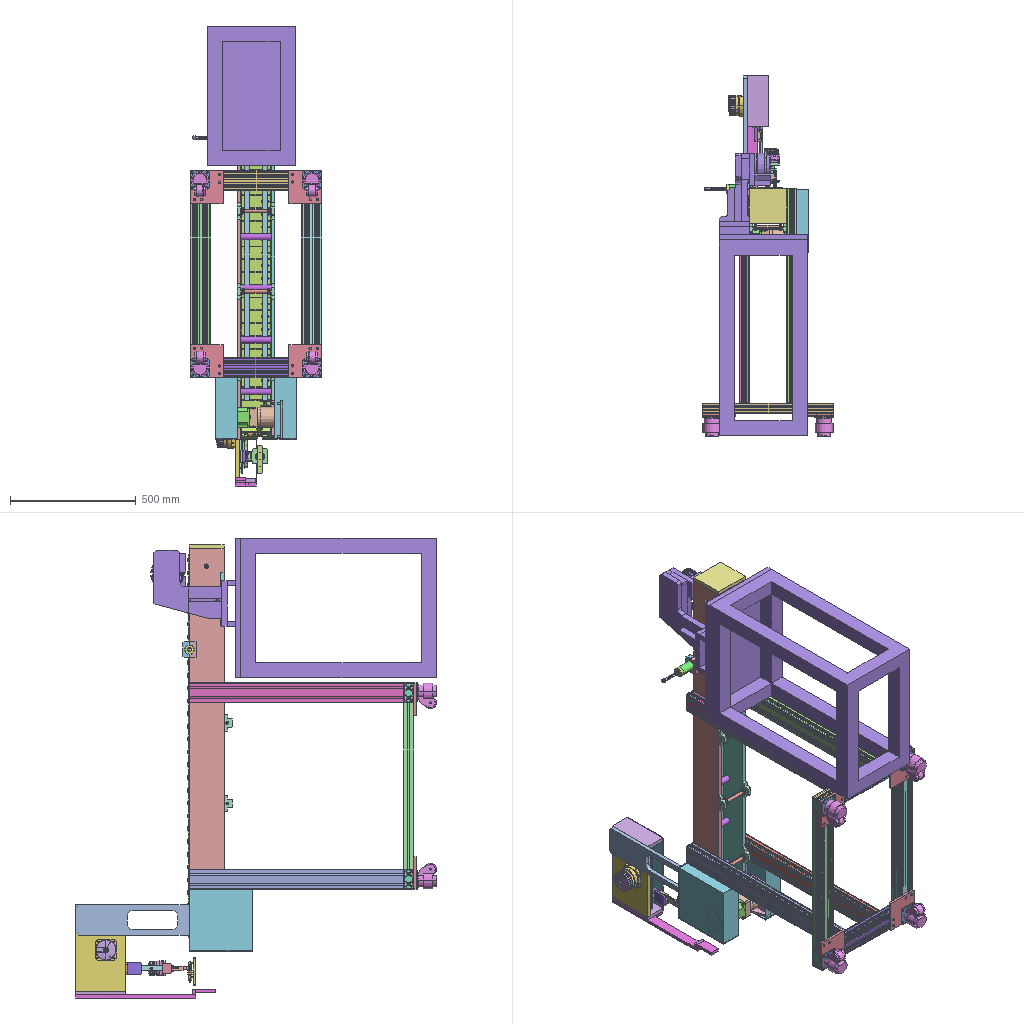Assembly | STEP file | 68 different items | 200 placed | box 524 x 1433 x 1827 mm
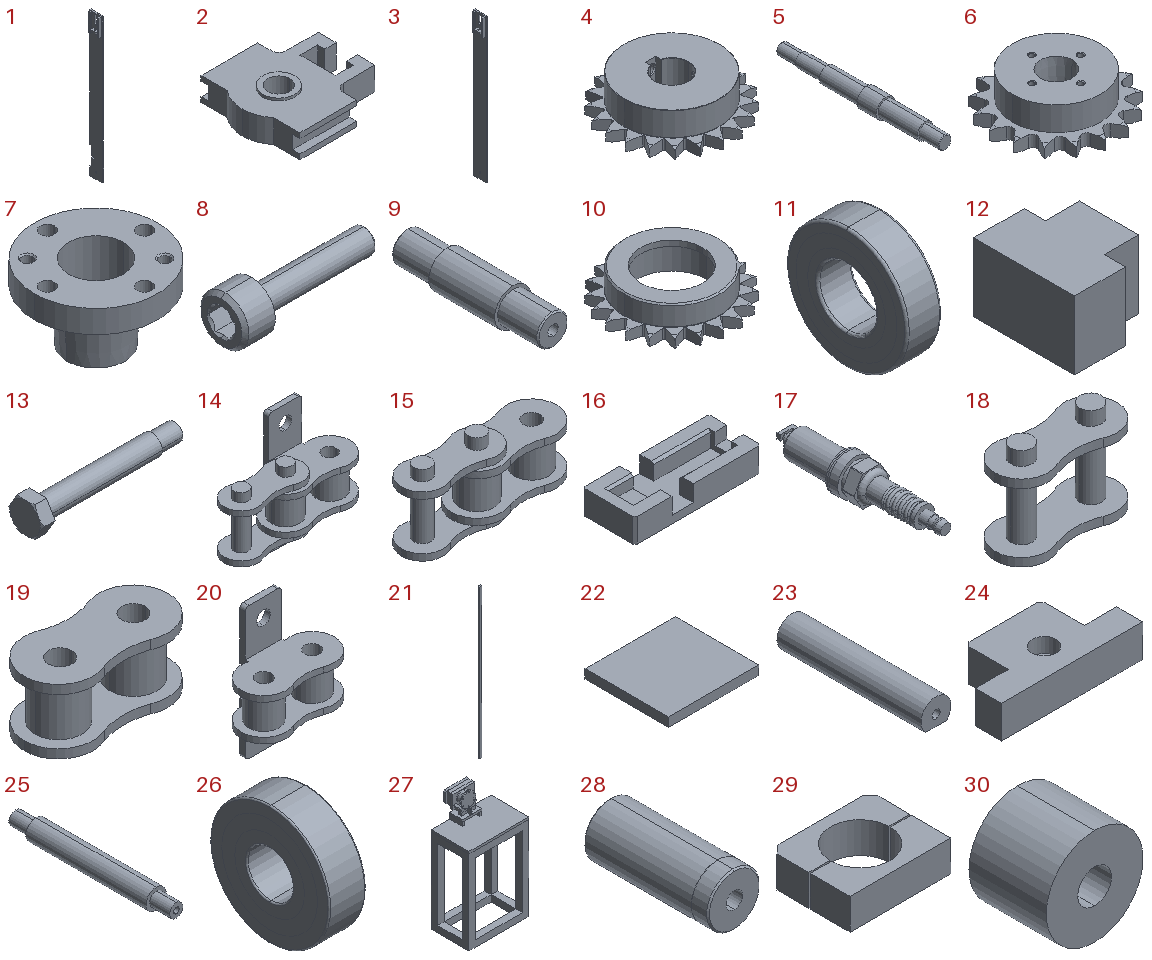Parts list (item | name | quantity | parent item | size | volume):
1 | PN_0020 | x1 | - | 50 x 139 x 1600 mm | 3436426 mm3
2 | UCT204 | x2 | - | 94 x 89 x 31 mm | 112461 mm3
3 | PN_0012 | x1 | - | 50 x 139 x 1600 mm | 3495566 mm3
4 | SP40B21_N_25_SP40B21-N-25 | x2 | - | 91.743 x 91.486 x 25 mm | 93110 mm3
5 | PN_0021 | x1 | - | 30 x 255 x 30 mm | 110798 mm3
6 | LFSP40B17_17_Asp | x2 | in LFSP40B17_17_A_LFSP40B17-17-A | 75.676 x 75.353 x 22 mm | 51808 mm3
7 | LFSP35B_17_boltbushing | x2 | in LFSP40B17_17_A_LFSP40B17-17-A | 38 x 38 x 23 mm | 6598 mm3
8 | LFSP35B17boltbolt | x8 | in LFSP40B17_17_A_LFSP40B17-17-A | 24 x 8 x 8 mm | 437.542 mm3
9 | PN_0023 | x1 | - | 30 x 120 x 30 mm | 67614 mm3
10 | PN_0022_SP40B21-N-25 | x2 | - | 91.743 x 91.486 x 22 mm | 50734 mm3
11 | 6205ZZ series deep groove ball bearing_6205ZZ | x2 | - | 15 x 52 x 52 mm | 22330 mm3
12 | PN_0024 | x2 | - | 26 x 31 x 21 mm | 12363 mm3
13 | PN_0025_M14x95 | x2 | - | 103.8 x 24.249 x 21 mm | 17342 mm3
14 | CHEL40Achain | x6 | in CHEL40A_4_CHEL40A-4 | 36.1 x 13.75 x 34.8 mm | 2522 mm3
15 | CHEL40Achain-2 | x4 | in CHEL40A_4_CHEL40A-4 | 36.1 x 11.7 x 17.55 mm | 2131 mm3
16 | PN_0002 | x33 | in PN_0001 | 116 x 48 x 22 mm | 82271 mm3
17 | FR8SES | x36 | in PN_0001, Assembly 2, PN_0030, PN_0045 | 18.6 x 85.1 x 18.6 mm | 9845 mm3
18 | CHEL40Achain-3 | x4 | - | 22.4 x 9.7 x 17.55 mm | 895.476 mm3
19 | CHEL40Achain-4 | x2 | - | 24.4 x 11.7 x 10.95 mm | 1235 mm3
20 | CHEL40Achain-5 | x2 | - | 24.4 x 13.75 x 34.8 mm | 1627 mm3
21 | PN_0026 | x2 | - | 20 x 16 x 1290 mm | 377295 mm3
22 | PN_0004 | x1 | - | 150 x 139 x 15 mm | 312750 mm3
23 | PN_0003 | x5 | - | 25 x 120 x 21.5 mm | 52408 mm3
24 | PN_0005 | x6 | - | 65 x 32 x 15 mm | 21213 mm3
25 | PN_0006 | x3 | - | 15 x 120 x 15 mm | 17905 mm3
26 | 6000ZZ series deep groove ball bearing_6000ZZ | x6 | - | 8 x 26 x 26 mm | 3330 mm3
27 | Wire-arranging machine schematic | x1 | in Assembly 2 | 555 x 350.2 x 1135 mm | 27799243 mm3
28 | PN_0007 | x1 | in PN_0027 | 38 x 97.6 x 38 mm | 92613 mm3
29 | PN_0008 | x1 | in PN_0027 | 65 x 52 x 20 mm | 43878 mm3
30 | PN_0011 | x1 | in PN_0027 | 10 x 8 x 10 mm | 476.737 mm3
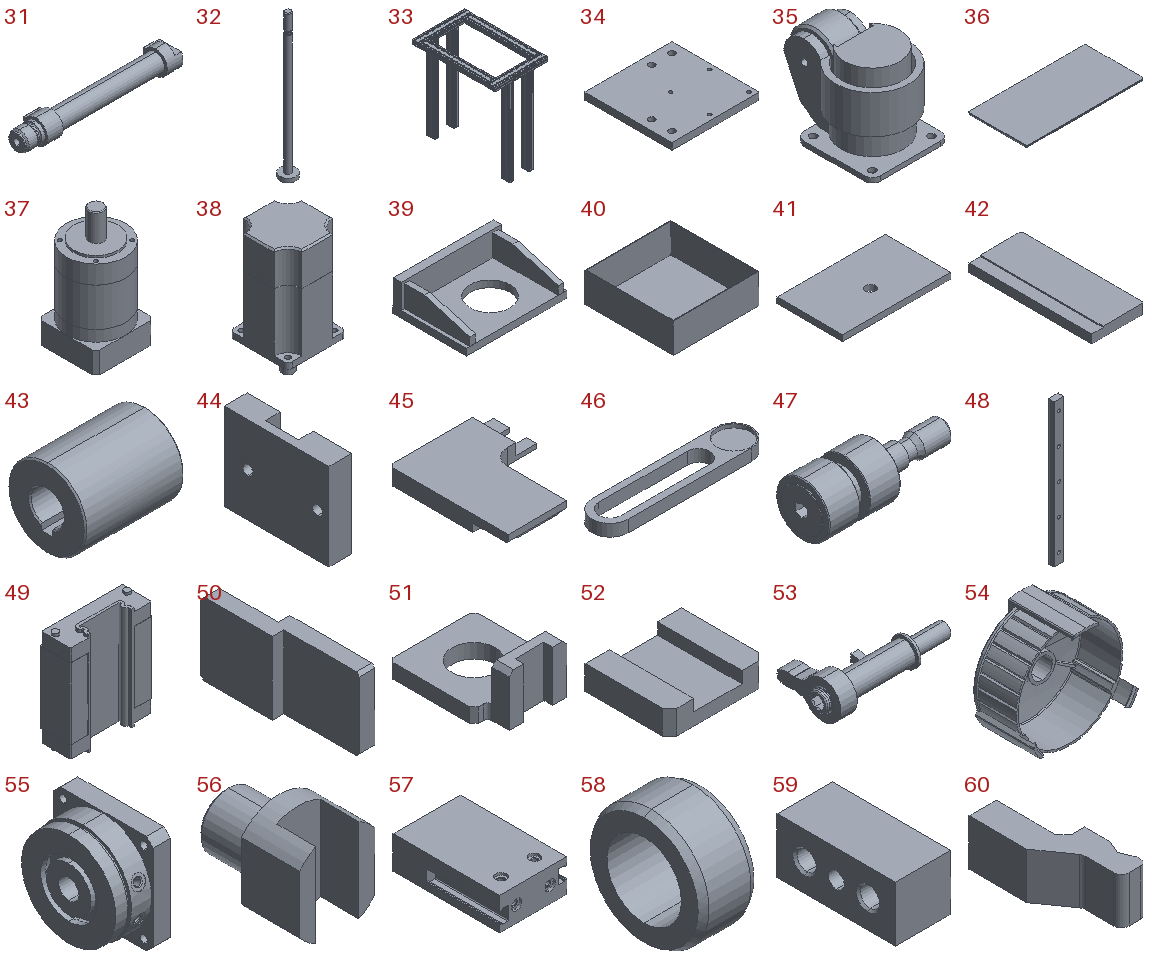31 | PN_0051 | x1 | in PN_0049 | 98 x 15 x 15 mm | 7309 mm3
32 | PN_0050 | x1 | in PN_0049 | 10 x 10 x 90 mm | 1287 mm3
33 | PN_0009 | x1 | in PN_0028 | 520 x 820 x 892 mm | 7509910 mm3
34 | PN_0010 | x4 | in PN_0028 | 130 x 130 x 10 mm | 165650 mm3
35 | FM wheel (3 in) | x4 | in PN_0028 | 74 x 103.967 x 80 mm | 304180 mm3
36 | Profile end cap | x8 | in PN_0028 | 80 x 40 x 2 mm | 6284 mm3
37 | PL80-40 | x1 | in Wire-arranging machine servo motor | 80 x 80 x 162 mm | 651730 mm3
38 | 1FL40-44-0AF21-0AA0 | x1 | in Wire-arranging machine servo motor | 80 x 80 x 173 mm | 725829 mm3
39 | PN_0013 | x1 | - | 150 x 110 x 46.5 mm | 242294 mm3
40 | PN_0014 | x2 | - | 247 x 253 x 86 mm | 291638 mm3
41 | PN_0031 | x1 | in PN_0030 | 330 x 200 x 18 mm | 1175277 mm3
42 | PN_0036 | x2 | in PN_0030 | 85 x 200 x 16 mm | 264736 mm3
43 | PN_0037 | x1 | in PN_0030 | 35.5 x 28 x 28 mm | 17402 mm3
44 | PN_0039 | x1 | in PN_0030 | 13 x 60 x 50 mm | 29683 mm3
45 | PN_0038 | x1 | in PN_0030 | 120 x 137 x 18 mm | 154666 mm3
46 | PN_0040 | x1 | in PN_0030 | 133.5 x 30 x 10 mm | 19376 mm3
47 | PN_0034 | x1 | in PN_0030 | 50 x 19 x 19 mm | 7855 mm3
48 | r_SEBZ20_280 | x2 | in PN_0030 | 20 x 11 x 280 mm | 56779 mm3
49 | b_SEZB20 | x2 | in PN_0030 | 40 x 15 x 50 mm | 22286 mm3
50 | PN_0041 | x1 | in PN_0030 | 17.5 x 95 x 47 mm | 46685 mm3
51 | PN_0015 | x1 | in PN_0030 | 59 x 74 x 35 mm | 41292 mm3
52 | PN_0017 | x1 | in PN_0030 | 40 x 35 x 10 mm | 10550 mm3
53 | PN_0052 | x1 | in DSM-12-180-P-A-B | 68.3 x 34.5 x 20 mm | 8759 mm3
54 | PN_0053 | x1 | in DSM-12-180-P-A-B | 55.4 x 33.7 x 57.2 mm | 9406 mm3
55 | PN_0054 | x1 | in DSM-12-180-P-A-B | 34 x 59 x 59 mm | 79656 mm3
56 | PN_0016 | x1 | in PN_0030 | 27 x 40 x 34 mm | 14723 mm3
57 | PN_0047 | x1 | in PN_0048 | 32 x 51 x 15.5 mm | 23128 mm3
58 | PN_0046 | x2 | in PN_0048 | 2.4 x 5 x 5 mm | 27.025 mm3
59 | - | x2 | in PN_0048 | 7 x 15 x 7 mm | 645.309 mm3
60 | PN_0018 | x2 | in PN_0030 | 12.5 x 33.5 x 12 mm | 2479 mm3
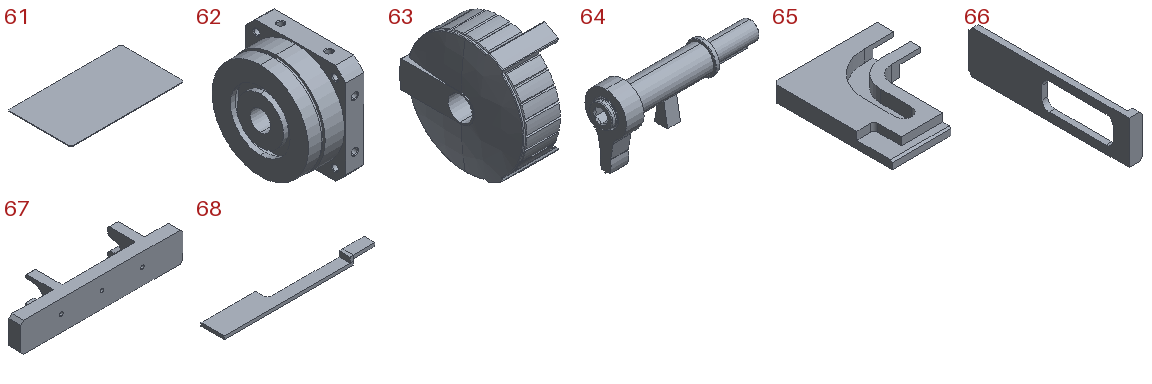61 | PN_0042 | x1 | in PN_0030 | 358 x 200 x 2 mm | 143100 mm3
62 | PN_0043 | x1 | in PN_0044 | 48.5 x 83 x 83 mm | 213563 mm3
63 | PN_0032 | x1 | in PN_0044 | 41.9 x 81.2 x 79.4 mm | 19535 mm3
64 | PN_0033 | x1 | in PN_0044 | 97.5 x 27 x 47.5 mm | 24592 mm3
65 | Mirror PN_0038 | x1 | in PN_0030 | 120 x 137 x 18 mm | 154666 mm3
66 | PN_0019 | x1 | - | 39.2 x 450 x 120 mm | 681574 mm3
67 | PN_0029 | x1 | in PN_0045 | 110 x 27 x 20 mm | 20647 mm3
68 | PN_0035 | x1 | - | 556.9 x 85 x 32 mm | 385323 mm3
Placements (level | parent | child | x y z in mm | rotation matrix by rows):
1 | subassembly 2 | PN_0020 | -9.547 61.103 0.0001 | 1 0 0 0 -1 0 0 0 -1
1 | subassembly 2 | UCT204 | -41.547 61.103 -1525.5 | 0 0 1 0 -1 0 1 0 0
1 | subassembly 2 | PN_0012 | 125.453 61.103 0.0001 | -1 0 0 0 1 0 0 0 -1
1 | subassembly 2 | UCT204 | 157.453 61.103 -1525.5 | 0 0 -1 0 1 0 1 0 -0
1 | subassembly 2 | SP40B21_N_25_SP40B21-N-25 | 97.953 61.103 -1525.5 | 0 0 -1 0 -1 0 -1 0 -0
1 | subassembly 2 | SP40B21_N_25_SP40B21-N-25 | 17.953 61.103 -1525.5 | 0 0 1 0 -1 0 1 0 0
1 | subassembly 2 | PN_0021 | -49.547 61.103 -1525.5 | 0 1 0 -0.5397 0 0.8419 0.8419 0 0.5397
1 | subassembly 2 | LFSP40B17_17_A_LFSP40B17-17-A | 174.453 61.103 -1525.5 | 0 0 -1 1.3e-05 -1 0 -1 -1.3e-05 -0
2 | LFSP40B17_17_A_LFSP40B17-17-A | LFSP40B17_17_Asp | -0.0 -0.0 -0.0 | -1 0 0 0 1 0 0 0 -1
2 | LFSP40B17_17_A_LFSP40B17-17-A | LFSP35B_17_boltbushing | 0.0 -0.0 -30.0 | -1 0 0 0 1 0 0 0 -1
2 | LFSP40B17_17_A_LFSP40B17-17-A | LFSP35B17boltbolt | -0.0 15.0 -35.0 | 0 0 1 0 -1 0 1 0 0
2 | LFSP40B17_17_A_LFSP40B17-17-A | LFSP35B17boltbolt | 15.0 0.0 -35.0 | 0 0 1 0 -1 0 1 0 0
2 | LFSP40B17_17_A_LFSP40B17-17-A | LFSP35B17boltbolt | 0.0 -15.0 -35.0 | 0 0 1 0 -1 0 1 0 0
2 | LFSP40B17_17_A_LFSP40B17-17-A | LFSP35B17boltbolt | -15.0 -0.0 -35.0 | 0 0 1 0 -1 0 1 0 0
1 | subassembly 2 | PN_0023 | -2.047 61.103 -70 | 0 1 0 1 0 1.3e-05 1.3e-05 0 -1
1 | subassembly 2 | PN_0022_SP40B21-N-25 | 17.953 61.103 -70 | 0 0 1 -1.3e-05 -1 0 1 -1.3e-05 0
1 | subassembly 2 | PN_0022_SP40B21-N-25 | 97.953 61.103 -70 | 0 0 -1 -0.9242 -0.3819 0 -0.3819 0.9242 -0
1 | subassembly 2 | 6205ZZ series deep groove ball bearing_6205ZZ | 87.453 61.103 -70 | 1 0 0 0 -1 1.3e-05 0 -1.3e-05 -1
1 | subassembly 2 | 6205ZZ series deep groove ball bearing_6205ZZ | 28.453 61.103 -70 | 1 0 0 0 -1 1.3e-05 0 -1.3e-05 -1
1 | subassembly 2 | PN_0024 | 136.453 76.603 -1490.5 | 0 0 1 0 -1 0 1 0 0
1 | subassembly 2 | PN_0024 | -41.547 76.603 -1490.5 | 0 0 1 0 -1 0 1 0 0
1 | subassembly 2 | PN_0025_M14x95 | 146.953 61.103 -1375.7 | 0 0 -1 0 -1 0 -1 0 -0
1 | subassembly 2 | PN_0025_M14x95 | -31.047 61.103 -1375.7 | 0 0 -1 0 -1 0 -1 0 -0
1 | subassembly 2 | CHEL40A_4_CHEL40A-4 | 94.353 103.708 -1500.1 | 0 0 1 0 1 0 -1 0 0
2 | CHEL40A_4_CHEL40A-4 | CHEL40Achain | -0.0 -0.0 -0.0 | 1 0 0 0 1 0 0 0 1
2 | CHEL40A_4_CHEL40A-4 | CHEL40Achain-2 | -25.4 -0.0 -0.0 | 1 0 0 0 1 0 0 0 1
2 | CHEL40A_4_CHEL40A-4 | CHEL40Achain | -50.8 -0.0 -0.0 | 1 0 0 0 1 0 0 0 1
2 | CHEL40A_4_CHEL40A-4 | CHEL40Achain-2 | -76.2 0.0 -0.0 | 1 0 0 0 1 0 0 0 1
2 | CHEL40A_4_CHEL40A-4 | CHEL40Achain | -101.6 0.0 -0.0 | 1 0 0 0 1 0 0 0 1
1 | subassembly 2 | PN_0001 | 57.953 111.608 -1519.15 | -1 0 0 0 0 1 0 1 0
2 | PN_0001 | PN_0002 | -0.0 -0.0 -0.0 | 1 0 0 0 1 0 0 0 1
2 | PN_0001 | FR8SES | -45.28 0.0 16.3 | 0 1 0 -1 0 0 0 0 1
1 | subassembly 2 | CHEL40A_4_CHEL40A-4 | 94.353 103.708 -1427.3 | 0 0 1 0 1 0 -1 0 0
2 | CHEL40A_4_CHEL40A-4 | CHEL40Achain | -0.0 -0.0 -0.0 | 1 0 0 0 1 0 0 0 1
2 | CHEL40A_4_CHEL40A-4 | CHEL40Achain-2 | -25.4 -0.0 -0.0 | 1 0 0 0 1 0 0 0 1
2 | CHEL40A_4_CHEL40A-4 | CHEL40Achain | -50.8 -0.0 -0.0 | 1 0 0 0 1 0 0 0 1
2 | CHEL40A_4_CHEL40A-4 | CHEL40Achain-2 | -76.2 0.0 -0.0 | 1 0 0 0 1 0 0 0 1
2 | CHEL40A_4_CHEL40A-4 | CHEL40Achain | -101.6 0.0 -0.0 | 1 0 0 0 1 0 0 0 1
1 | subassembly 2 | PN_0001 | 57.953 111.608 -1468.35 | -1 0 0 0 0 1 0 1 0
2 | PN_0001 | PN_0002 | -0.0 -0.0 -0.0 | 1 0 0 0 1 0 0 0 1
2 | PN_0001 | FR8SES | -45.28 0.0 16.3 | 0 1 0 -1 0 0 0 0 1
1 | subassembly 2 | PN_0001 | 57.953 111.608 -1417.55 | -1 0 0 0 0 1 0 1 0
2 | PN_0001 | PN_0002 | -0.0 -0.0 -0.0 | 1 0 0 0 1 0 0 0 1
2 | PN_0001 | FR8SES | -45.28 0.0 16.3 | 0 1 0 -1 0 0 0 0 1
1 | subassembly 2 | CHEL40Achain-3 | 94.353 103.708 -1525.5 | 0 0 -1 -0.149 -0.9888 0 -0.9888 0.149 -0
1 | subassembly 2 | CHEL40Achain-4 | 94.353 107.326 -1526.616 | 0 0 -1 -0.4339 -0.901 0 -0.901 0.4339 -0
1 | subassembly 2 | CHEL40Achain-3 | 94.353 76.669 -1565.16 | 0 0 -1 -0.9749 -0.2225 0 -0.2225 0.9749 -0
1 | subassembly 2 | CHEL40Achain-3 | 94.353 96.305 -1549.5 | 0 0 -1 -0.6802 -0.7331 0 -0.7331 0.6802 -0
1 | subassembly 2 | CHEL40Achain-5 | 94.353 65.671 -1571.511 | 0 0 -1 0.866 0.5 0 0.5 -0.866 -0
1 | subassembly 2 | CHEL40Achain-4 | 94.353 76.951 -1568.935 | 0 0 -1 -0.9972 0.07473 0 0.07473 0.9972 -0
1 | subassembly 2 | CHEL40Achain-5 | 91.353 19.942 -1546.56 | 0 0 -1 0.7818 -0.6235 0 -0.6235 -0.7818 -0
1 | subassembly 2 | CHEL40Achain-3 | 94.353 51.623 -1567.037 | 0 0 -1 -0.9309 0.3653 0 0.3653 0.9309 -0
1 | subassembly 2 | PN_0001 | 57.953 86.118 -1568.826 | -1 0 0 0 0.866 0.5 0 0.5 -0.866
2 | PN_0001 | PN_0002 | -0.0 -0.0 -0.0 | 1 0 0 0 1 0 0 0 1
2 | PN_0001 | FR8SES | -45.28 0.0 16.3 | 0 1 0 -1 0 0 0 0 1
1 | subassembly 2 | PN_0026 | 84.353 83.733 -1445 | 1 0 0 0 1 0 0 0 1
1 | subassembly 2 | PN_0026 | 11.553 83.733 -1445 | 1 0 0 0 1 0 0 0 1
1 | subassembly 2 | PN_0001 | 57.953 111.608 -1366.75 | -1 0 0 0 0 1 0 1 0
2 | PN_0001 | PN_0002 | -0.0 -0.0 -0.0 | 1 0 0 0 1 0 0 0 1
2 | PN_0001 | FR8SES | -45.28 0.0 16.3 | 0 1 0 -1 0 0 0 0 1
1 | subassembly 2 | PN_0001 | 57.953 111.608 -1315.95 | -1 0 0 0 0 1 0 1 0
2 | PN_0001 | PN_0002 | -0.0 -0.0 -0.0 | 1 0 0 0 1 0 0 0 1
2 | PN_0001 | FR8SES | -45.28 0.0 16.3 | 0 1 0 -1 0 0 0 0 1
1 | subassembly 2 | PN_0001 | 57.953 111.608 -1265.15 | -1 0 0 0 0 1 0 1 0
2 | PN_0001 | PN_0002 | -0.0 -0.0 -0.0 | 1 0 0 0 1 0 0 0 1
2 | PN_0001 | FR8SES | -45.28 0.0 16.3 | 0 1 0 -1 0 0 0 0 1
1 | subassembly 2 | PN_0001 | 57.953 111.608 -1214.35 | -1 0 0 0 0 1 0 1 0
2 | PN_0001 | PN_0002 | -0.0 -0.0 -0.0 | 1 0 0 0 1 0 0 0 1
2 | PN_0001 | FR8SES | -45.28 0.0 16.3 | 0 1 0 -1 0 0 0 0 1
1 | subassembly 2 | PN_0001 | 57.953 111.608 -1163.55 | -1 0 0 0 0 1 0 1 0
2 | PN_0001 | PN_0002 | -0.0 -0.0 -0.0 | 1 0 0 0 1 0 0 0 1
2 | PN_0001 | FR8SES | -45.28 0.0 16.3 | 0 1 0 -1 0 0 0 0 1
1 | subassembly 2 | PN_0001 | 57.953 111.608 -1112.75 | -1 0 0 0 0 1 0 1 0
2 | PN_0001 | PN_0002 | -0.0 -0.0 -0.0 | 1 0 0 0 1 0 0 0 1
2 | PN_0001 | FR8SES | -45.28 0.0 16.3 | 0 1 0 -1 0 0 0 0 1
1 | subassembly 2 | PN_0001 | 57.953 111.608 -1061.95 | -1 0 0 0 0 1 0 1 0
2 | PN_0001 | PN_0002 | -0.0 -0.0 -0.0 | 1 0 0 0 1 0 0 0 1
2 | PN_0001 | FR8SES | -45.28 0.0 16.3 | 0 1 0 -1 0 0 0 0 1
1 | subassembly 2 | PN_0001 | 57.953 111.608 -1011.15 | -1 0 0 0 0 1 0 1 0
2 | PN_0001 | PN_0002 | -0.0 -0.0 -0.0 | 1 0 0 0 1 0 0 0 1
2 | PN_0001 | FR8SES | -45.28 0.0 16.3 | 0 1 0 -1 0 0 0 0 1
1 | subassembly 2 | PN_0001 | 57.953 111.608 -960.35 | -1 0 0 0 0 1 0 1 0
2 | PN_0001 | PN_0002 | -0.0 -0.0 -0.0 | 1 0 0 0 1 0 0 0 1
2 | PN_0001 | FR8SES | -45.28 0.0 16.3 | 0 1 0 -1 0 0 0 0 1
1 | subassembly 2 | PN_0001 | 57.953 111.608 -909.55 | -1 0 0 0 0 1 0 1 0
2 | PN_0001 | PN_0002 | -0.0 -0.0 -0.0 | 1 0 0 0 1 0 0 0 1
2 | PN_0001 | FR8SES | -45.28 0.0 16.3 | 0 1 0 -1 0 0 0 0 1
1 | subassembly 2 | PN_0001 | 57.953 111.608 -858.75 | -1 0 0 0 0 1 0 1 0
2 | PN_0001 | PN_0002 | -0.0 -0.0 -0.0 | 1 0 0 0 1 0 0 0 1
2 | PN_0001 | FR8SES | -45.28 0.0 16.3 | 0 1 0 -1 0 0 0 0 1
1 | subassembly 2 | PN_0001 | 57.953 111.608 -807.95 | -1 0 0 0 0 1 0 1 0
2 | PN_0001 | PN_0002 | -0.0 -0.0 -0.0 | 1 0 0 0 1 0 0 0 1
2 | PN_0001 | FR8SES | -45.28 0.0 16.3 | 0 1 0 -1 0 0 0 0 1
1 | subassembly 2 | PN_0001 | 57.953 111.608 -757.15 | -1 0 0 0 0 1 0 1 0
2 | PN_0001 | PN_0002 | -0.0 -0.0 -0.0 | 1 0 0 0 1 0 0 0 1
2 | PN_0001 | FR8SES | -45.28 0.0 16.3 | 0 1 0 -1 0 0 0 0 1
1 | subassembly 2 | PN_0001 | 57.953 111.608 -706.35 | -1 0 0 0 0 1 0 1 0
2 | PN_0001 | PN_0002 | -0.0 -0.0 -0.0 | 1 0 0 0 1 0 0 0 1
2 | PN_0001 | FR8SES | -45.28 0.0 16.3 | 0 1 0 -1 0 0 0 0 1
1 | subassembly 2 | PN_0001 | 57.953 111.608 -655.55 | -1 0 0 0 0 1 0 1 0
2 | PN_0001 | PN_0002 | -0.0 -0.0 -0.0 | 1 0 0 0 1 0 0 0 1
2 | PN_0001 | FR8SES | -45.28 0.0 16.3 | 0 1 0 -1 0 0 0 0 1
1 | subassembly 2 | PN_0001 | 57.953 111.608 -604.75 | -1 0 0 0 0 1 0 1 0
2 | PN_0001 | PN_0002 | -0.0 -0.0 -0.0 | 1 0 0 0 1 0 0 0 1
2 | PN_0001 | FR8SES | -45.28 0.0 16.3 | 0 1 0 -1 0 0 0 0 1
1 | subassembly 2 | PN_0001 | 57.953 111.608 -553.95 | -1 0 0 0 0 1 0 1 0
2 | PN_0001 | PN_0002 | -0.0 -0.0 -0.0 | 1 0 0 0 1 0 0 0 1
2 | PN_0001 | FR8SES | -45.28 0.0 16.3 | 0 1 0 -1 0 0 0 0 1
1 | subassembly 2 | PN_0001 | 57.953 111.608 -503.15 | -1 0 0 0 0 1 0 1 0
2 | PN_0001 | PN_0002 | -0.0 -0.0 -0.0 | 1 0 0 0 1 0 0 0 1
2 | PN_0001 | FR8SES | -45.28 0.0 16.3 | 0 1 0 -1 0 0 0 0 1
1 | subassembly 2 | PN_0004 | 57.953 60.103 15 | 1 0 0 0 -1 0 0 0 -1
1 | subassembly 2 | PN_0003 | -2.047 74.733 -1410 | 0 1 0 0 0 -1 -1 0 0
1 | subassembly 2 | PN_0003 | -2.047 74.733 -1205 | 0 1 0 0 0 -1 -1 0 0
1 | subassembly 2 | PN_0003 | -2.047 74.733 -1000 | 0 1 0 0 0 -1 -1 0 0
1 | subassembly 2 | PN_0003 | -2.047 74.733 -795 | 0 1 0 0 0 -1 -1 0 0
1 | subassembly 2 | PN_0003 | -2.047 74.733 -590 | 0 1 0 0 0 -1 -1 0 0
1 | subassembly 2 | PN_0005 | -2.047 -9.397 -1300 | 0 0 -1 0 -1 0 -1 0 -0
1 | subassembly 2 | PN_0005 | 117.953 -9.397 -1365 | 0 0 1 0 -1 0 1 0 0
1 | subassembly 2 | PN_0006 | 117.953 -22.397 -1332.5 | 0 -1 0 -1 0 1.3e-05 -1.3e-05 0 -1
1 | subassembly 2 | 6000ZZ series deep groove ball bearing_6000ZZ | 106.953 -22.397 -1332.5 | 1 0 0 0 -1 1.3e-05 0 -1.3e-05 -1
1 | subassembly 2 | 6000ZZ series deep groove ball bearing_6000ZZ | 8.953 -22.397 -1332.5 | 1 0 0 0 -1 1.3e-05 0 -1.3e-05 -1
1 | subassembly 2 | 6000ZZ series deep groove ball bearing_6000ZZ | 8.953 -22.397 -1012.5 | 1 0 0 0 -1 1.3e-05 0 -1.3e-05 -1
1 | subassembly 2 | 6000ZZ series deep groove ball bearing_6000ZZ | 8.953 -22.397 -692.5 | 1 0 0 0 -1 1.3e-05 0 -1.3e-05 -1
1 | subassembly 2 | 6000ZZ series deep groove ball bearing_6000ZZ | 106.953 -22.397 -1012.5 | 1 0 0 0 -1 1.3e-05 0 -1.3e-05 -1
1 | subassembly 2 | 6000ZZ series deep groove ball bearing_6000ZZ | 106.953 -22.397 -692.5 | 1 0 0 0 -1 1.3e-05 0 -1.3e-05 -1
1 | subassembly 2 | PN_0006 | 117.953 -22.397 -1012.5 | 0 -1 0 -1 0 1.3e-05 -1.3e-05 0 -1
1 | subassembly 2 | PN_0006 | 117.953 -22.397 -692.5 | 0 -1 0 -1 0 1.3e-05 -1.3e-05 0 -1
1 | subassembly 2 | PN_0005 | 117.953 -9.397 -1045 | 0 0 1 0 -1 0 1 0 0
1 | subassembly 2 | PN_0005 | 117.953 -9.397 -725 | 0 0 1 0 -1 0 1 0 0
1 | subassembly 2 | PN_0005 | -2.047 -9.397 -980 | 0 0 -1 0 -1 0 -1 0 -0
1 | subassembly 2 | PN_0005 | -2.047 -9.397 -660 | 0 0 -1 0 -1 0 -1 0 -0
1 | subassembly 2 | Assembly 2 | 65.282 -285.2 -269.877 | 0 -1 0 0 0 1 -1 0 0
2 | Assembly 2 | Wire-arranging machine schematic | -34.227 26.198 -567.392 | 1 0 0 0 1 0 0 0 1
2 | Assembly 2 | PN_0001 | -173.127 7.329 396.808 | 0 -1 0 1 0 0 0 0 1
3 | PN_0001 | PN_0002 | -0.0 -0.0 -0.0 | 1 0 0 0 1 0 0 0 1
3 | PN_0001 | FR8SES | -45.28 0.0 16.3 | 0 1 0 -1 0 0 0 0 1
2 | Assembly 2 | FR8SES | -169.127 -37.951 443.458 | 1 0 0 0 1 0 0 0 1
1 | subassembly 2 | PN_0001 | 57.953 29.912 -1564.616 | -1 0 0 0 0.7819 -0.6234 0 -0.6234 -0.7819
2 | PN_0001 | PN_0002 | -0.0 -0.0 -0.0 | 1 0 0 0 1 0 0 0 1
2 | PN_0001 | FR8SES | -45.28 0.0 16.3 | 0 1 0 -1 0 0 0 0 1
1 | subassembly 2 | PN_0001 | 57.953 111.608 -452.35 | -1 0 0 0 0 1 0 1 0
2 | PN_0001 | PN_0002 | -0.0 -0.0 -0.0 | 1 0 0 0 1 0 0 0 1
2 | PN_0001 | FR8SES | -45.28 0.0 16.3 | 0 1 0 -1 0 0 0 0 1
1 | subassembly 2 | PN_0001 | 57.953 111.608 -401.55 | -1 0 0 0 0 1 0 1 0
2 | PN_0001 | PN_0002 | -0.0 -0.0 -0.0 | 1 0 0 0 1 0 0 0 1
2 | PN_0001 | FR8SES | -45.28 0.0 16.3 | 0 1 0 -1 0 0 0 0 1
1 | subassembly 2 | PN_0001 | 57.953 111.608 -350.75 | -1 0 0 0 0 1 0 1 0
2 | PN_0001 | PN_0002 | -0.0 -0.0 -0.0 | 1 0 0 0 1 0 0 0 1
2 | PN_0001 | FR8SES | -45.28 0.0 16.3 | 0 1 0 -1 0 0 0 0 1
1 | subassembly 2 | PN_0001 | 57.953 111.608 -299.95 | -1 0 0 0 0 1 0 1 0
2 | PN_0001 | PN_0002 | -0.0 -0.0 -0.0 | 1 0 0 0 1 0 0 0 1
2 | PN_0001 | FR8SES | -45.28 0.0 16.3 | 0 1 0 -1 0 0 0 0 1
1 | subassembly 2 | PN_0001 | 57.953 111.608 -249.15 | -1 0 0 0 0 1 0 1 0
2 | PN_0001 | PN_0002 | -0.0 -0.0 -0.0 | 1 0 0 0 1 0 0 0 1
2 | PN_0001 | FR8SES | -45.28 0.0 16.3 | 0 1 0 -1 0 0 0 0 1
1 | subassembly 2 | PN_0001 | 57.953 111.608 -198.35 | -1 0 0 0 0 1 0 1 0
2 | PN_0001 | PN_0002 | -0.0 -0.0 -0.0 | 1 0 0 0 1 0 0 0 1
2 | PN_0001 | FR8SES | -45.28 0.0 16.3 | 0 1 0 -1 0 0 0 0 1
1 | subassembly 2 | PN_0001 | 57.953 111.608 -147.55 | -1 0 0 0 0 1 0 1 0
2 | PN_0001 | PN_0002 | -0.0 -0.0 -0.0 | 1 0 0 0 1 0 0 0 1
2 | PN_0001 | FR8SES | -45.28 0.0 16.3 | 0 1 0 -1 0 0 0 0 1
1 | subassembly 2 | PN_0001 | 57.953 111.608 -96.75 | -1 0 0 0 0 1 0 1 0
2 | PN_0001 | PN_0002 | -0.0 -0.0 -0.0 | 1 0 0 0 1 0 0 0 1
2 | PN_0001 | FR8SES | -45.28 0.0 16.3 | 0 1 0 -1 0 0 0 0 1
1 | subassembly 2 | PN_0001 | 57.953 111.608 -45.95 | -1 0 0 0 0 1 0 1 0
2 | PN_0001 | PN_0002 | -0.0 -0.0 -0.0 | 1 0 0 0 1 0 0 0 1
2 | PN_0001 | FR8SES | -45.28 0.0 16.3 | 0 1 0 -1 0 0 0 0 1
1 | subassembly 2 | PN_0027 | -61.974 132.786 -431.6 | 0 1 0 0.1602 0 -0.9871 -0.9871 0 -0.1602
2 | PN_0027 | PN_0007 | -30.444 -33.073 -0.0 | 1 0 0 0 1 0 0 0 1
2 | PN_0027 | PN_0008 | -30.444 24.927 0.0 | 0.9871 0.1602 0 0 0 1 0.1602 -0.9871 0
2 | PN_0027 | PN_0011 | -30.444 52.427 -0.0 | 1 0 0 0 1 0 0 0 1
2 | PN_0027 | PN_0049 | -30.444 -33.173 0.0 | 0.9871 0.1602 0 0 0 1 0.1602 -0.9871 0
3 | PN_0049 | PN_0051 | -0.0 -0.0 -0.0 | 0 0 1 0 1 0 -1 0 0
3 | PN_0049 | PN_0050 | -0.0 0.0 -0.0 | -1 0 0 0 -1 0 0 0 1
1 | subassembly 2 | PN_0028 | 183.184 129.408 -915.68 | 1 0 0 0 0 -1 0 1 -0
2 | PN_0028 | PN_0009 | -30.231 -397.47 0.0 | 1 0 0 0 1 0 0 0 1
2 | PN_0028 | PN_0010 | -364.948 349.902 892.0 | -1 0 0 0 -1 0 0 0 1
2 | PN_0028 | PN_0010 | 102.141 362.247 892.0 | 0 -1 0 1 0 0 0 0 1
2 | PN_0028 | PN_0010 | -352.603 -417.187 892.0 | 0 1 0 -1 0 0 0 0 1
2 | PN_0028 | PN_0010 | 114.487 -404.842 892.0 | 1 0 0 0 1 0 0 0 1
2 | PN_0028 | FM wheel (3 in) | 98.269 -400.97 902.0 | 1 0 0 0 1 0 0 0 1
2 | PN_0028 | FM wheel (3 in) | 97.269 346.03 902.0 | -1 0 0 0 -1 0 0 0 1
2 | PN_0028 | FM wheel (3 in) | -347.731 -400.97 902.0 | 1 0 0 0 1 0 0 0 1
2 | PN_0028 | FM wheel (3 in) | -348.731 346.03 902.0 | -1 0 0 0 -1 0 0 0 1
2 | PN_0028 | Profile end cap | -220.231 342.53 -2.0 | 0 1 0 -1 0 0 0 0 1
2 | PN_0028 | Profile end cap | -30.231 342.53 -2.0 | 0 1 0 -1 0 0 0 0 1
2 | PN_0028 | Profile end cap | -220.231 -397.47 -2.0 | 0 1 0 -1 0 0 0 0 1
2 | PN_0028 | Profile end cap | -30.231 -397.47 -2.0 | 0 1 0 -1 0 0 0 0 1
2 | PN_0028 | Profile end cap | -387.231 342.53 872.0 | 0 0 1 -1 0 0 0 -1 0
2 | PN_0028 | Profile end cap | 136.769 342.53 872.0 | 0 0 -1 -1 0 0 0 1 -0
2 | PN_0028 | Profile end cap | 136.769 -397.47 872.0 | 0 0 -1 -1 0 0 0 1 -0
2 | PN_0028 | Profile end cap | -387.231 -397.47 872.0 | 0 0 1 -1 0 0 0 -1 0
1 | subassembly 2 | Wire-arranging machine servo motor | 32.453 -72.079 -1510.448 | 0 0 1 0.001151 1 0 -1 0.001151 0
2 | Wire-arranging machine servo motor | PL80-40 | 1.655 2.68 0.0 | 1 0 0 0 1 0 0 0 1
2 | Wire-arranging machine servo motor | 1FL40-44-0AF21-0AA0 | 1.655 2.68 0.0 | -1 0 0 0 1 0 0 0 -1
1 | subassembly 2 | LFSP40B17_17_A_LFSP40B17-17-A | 174.453 -69.397 -1512.1 | 0 0 -1 -0.09189 -0.9958 0 -0.9958 0.09189 -0
2 | LFSP40B17_17_A_LFSP40B17-17-A | LFSP40B17_17_Asp | -0.0 -0.0 -0.0 | -1 0 0 0 1 0 0 0 -1
2 | LFSP40B17_17_A_LFSP40B17-17-A | LFSP35B_17_boltbushing | 0.0 -0.0 -30.0 | -1 0 0 0 1 0 0 0 -1
2 | LFSP40B17_17_A_LFSP40B17-17-A | LFSP35B17boltbolt | -0.0 15.0 -35.0 | 0 0 1 0 -1 0 1 0 0
2 | LFSP40B17_17_A_LFSP40B17-17-A | LFSP35B17boltbolt | 15.0 0.0 -35.0 | 0 0 1 0 -1 0 1 0 0
2 | LFSP40B17_17_A_LFSP40B17-17-A | LFSP35B17boltbolt | 0.0 -15.0 -35.0 | 0 0 1 0 -1 0 1 0 0
2 | LFSP40B17_17_A_LFSP40B17-17-A | LFSP35B17boltbolt | -15.0 -0.0 -35.0 | 0 0 1 0 -1 0 1 0 0
1 | subassembly 2 | PN_0013 | 164.453 -64.297 -1522.1 | 0 0 -1 0 1 0 1 0 -0
1 | subassembly 2 | PN_0014 | 218.953 3.103 -1476.5 | 0 0 -1 0 1 0 1 0 -0
1 | subassembly 2 | PN_0014 | -103.047 3.103 -1476.5 | 0 0 1 0 1 0 -1 0 0
1 | subassembly 2 | PN_0030 | -7.247 470.095 -1585.859 | 0 0 -1 0 1 0 1 0 -0
2 | PN_0030 | PN_0031 | -8.291 10.05 0.0 | 1 0 0 0 1 0 0 0 1
2 | PN_0030 | PN_0036 | -187.291 10.05 -24.5 | 0 0 1 0 1 0 -1 0 -0
2 | PN_0030 | PN_0036 | 170.709 10.05 -24.5 | 0 0 -1 0 -1 0 -1 0 0
2 | PN_0030 | PN_0037 | -8.291 -9.95 18.0 | 0 -0.9999 0.01176 0 0.01176 0.9999 -1 0 0
2 | PN_0030 | PN_0039 | -8.291 0.05 19.5 | 0 0 1 0 1 0 -1 0 -0
2 | PN_0030 | PN_0038 | -69.291 22.05 -18.0 | 1 0 0 0 1 0 0 0 1
2 | PN_0030 | PN_0040 | -111.791 -9.95 -31.0 | 1 0 0 0 1 0 0 0 1
2 | PN_0030 | PN_0034 | -70.743 54.104 20.0 | 0 0.9854 -0.17 0 -0.17 -0.9854 -1 0 0
2 | PN_0030 | r_SEBZ20_280 | -81.791 10.05 -42.5 | 1 0 0 0 0 -1 0 1 -0
2 | PN_0030 | b_SEZB20 | -81.791 -151.45 -37.4 | 1 0 0 0 0 -1 0 1 -0
2 | PN_0030 | PN_0041 | -58.291 -149.95 -30.0 | 0 0 -1 0 1 0 1 0 0
2 | PN_0030 | PN_0015 | -81.791 -234.95 -42.5 | -1 0 0 0 0 -1 0 -1 -0
2 | PN_0030 | PN_0017 | -81.791 -252.45 -26.3 | -1 0 0 0 1 0 0 0 -1
2 | PN_0030 | DSM-12-180-P-A-B | -84.94 -226.292 -81.457 | 0 0.9896 -0.1438 -1 0 0 0 0.1438 0.9896
3 | DSM-12-180-P-A-B | PN_0052 | 8.658 3.182 -0.0 | 1 0 0 0 1 0 0 0 1
3 | DSM-12-180-P-A-B | PN_0053 | -22.342 3.182 -0.0 | 0 -1 0 1 0 0 0 0 1
3 | DSM-12-180-P-A-B | PN_0054 | 8.658 3.182 0.0 | 1 0 0 0 0.9896 0.1438 0 -0.1438 0.9896
2 | PN_0030 | PN_0016 | -81.791 -279.45 -81.0 | -1 0 0 0 1 0 0 0 -1
2 | PN_0030 | PN_0048 | -81.791 -265.45 -81.0 | 0 0 -1 0 -1 0 -1 0 0
3 | PN_0048 | PN_0047 | 0.0 -0.0 -0.0 | 1 0 0 0 1 0 0 0 1
3 | PN_0048 | PN_0046 | -8.0 1.2 -0.0 | 0 0 1 -1 0 0 0 -1 0
3 | PN_0048 | PN_0046 | 8.0 1.2 -0.0 | 0 0 1 -1 0 0 0 -1 0
3 | PN_0048 | subassembly 3 | -7.9 51.0 -0.0 | -1 0 0 0 1 0 0 0 -1
3 | PN_0048 | subassembly 3 | 7.9 51.0 -0.0 | 1 0 0 0 1 0 0 0 1
2 | PN_0030 | PN_0018 | -75.791 -350.15 -100.9 | 0 0 -1 0 1 0 1 0 0
2 | PN_0030 | PN_0018 | -87.791 -350.15 -61.1 | 0 0 1 0 1 0 -1 0 -0
2 | PN_0030 | PN_0042 | -8.291 10.05 -69.0 | 1 0 0 0 1 0 0 0 1
2 | PN_0030 | FR8SES | -52.311 -344.15 -81.0 | 0 -1 0 0 0 -1 1 0 0
2 | PN_0030 | PN_0044 | -8.291 -14.366 27.373 | 0 0 1 0 1 0 -1 0 -0
3 | PN_0044 | PN_0043 | 9.373 4.416 -0.0 | 1 0 0 0 1 0 0 0 1
3 | PN_0044 | PN_0032 | 9.373 4.416 -0.0 | 1 0 0 0 1 0 0 0 1
3 | PN_0044 | PN_0033 | 9.373 4.416 -0.0 | 1 0 0 0 1 0 0 0 1
2 | PN_0030 | r_SEBZ20_280 | 131.709 -74.95 0.0 | 0 0 -1 1 0 0 0 -1 0
2 | PN_0030 | b_SEZB20 | -56.791 -74.95 -5.1 | 0 0 1 -1 0 0 0 -1 -0
2 | PN_0030 | Mirror PN_0038 | 52.709 22.05 -18.0 | -1 0 0 0 1 0 0 0 -1
1 | subassembly 2 | PN_0019 | -41.247 129.603 -1535.15 | 1 0 0 0 1 0 0 0 1
1 | subassembly 2 | PN_0045 | 83.753 114.102 -1672.606 | 0 0 -1 0 1 0 1 0 -0
2 | PN_0045 | PN_0029 | -26.463 -2.157 -0.0 | 1 0 0 0 1 0 0 0 1
2 | PN_0045 | FR8SES | 34.437 11.843 10.0 | 0 -1 0 0.3058 0 0.9521 -0.9521 0 0.3058
1 | subassembly 2 | PN_0035 | 17.253 341.645 -1785.15 | 0 1 0 -1 0 0 0 0 1